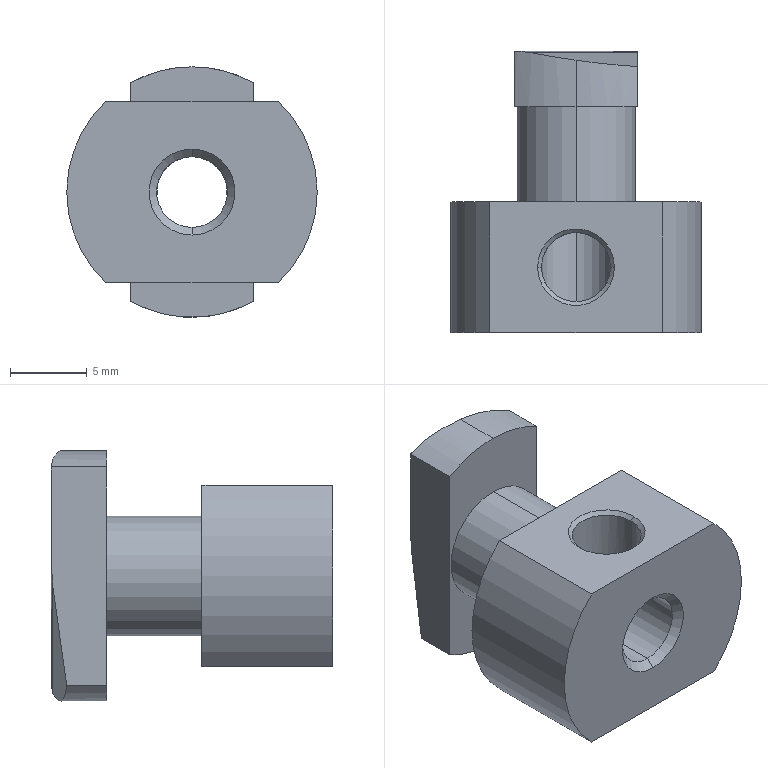Part | SolidWorks | features BaseBody 1 | 1 solid | 27 faces | box 16.3 x 18.3 x 16.3 mm | volume 1833 mm3 | cylinder 13 | plane 10 | cone 4 | commonest cylinder face diameters 16.3 x5 4.5 x2 4.6 x2 7.8 x2 10 x2
STEP:
#1=CARTESIAN_POINT('',(0.,-8.,2.3));
#2=VERTEX_POINT('',#1);
#3=CARTESIAN_POINT('',(0.,-8.,-2.3));
#4=VERTEX_POINT('',#3);
#5=CARTESIAN_POINT('',(0.,-8.,0.));
#6=DIRECTION('',(0.,-1.,0.));
#7=DIRECTION('',(0.,0.,-1.));
#8=AXIS2_PLACEMENT_3D('',#5,#6,#7);
#9=CIRCLE('',#8,2.3);
#10=EDGE_CURVE('',#2,#4,#9,.T.);
#11=ORIENTED_EDGE('',*,*,#10,.F.);
#12=CARTESIAN_POINT('',(0.,-8.5,2.8));
#13=VERTEX_POINT('',#12);
#14=CARTESIAN_POINT('',(0.,-8.5,2.8));
#15=DIRECTION('',(0.,-0.7071,0.7071));
#16=VECTOR('',#15,1000.);
#17=LINE('',#14,#16);
#18=EDGE_CURVE('',#2,#13,#17,.T.);
#19=ORIENTED_EDGE('',*,*,#18,.T.);
#20=CARTESIAN_POINT('',(0.,-8.5,-2.8));
#21=VERTEX_POINT('',#20);
#22=CARTESIAN_POINT('',(0.,-8.5,0.));
#23=DIRECTION('',(0.,-1.,0.));
#24=DIRECTION('',(0.,0.,-1.));
#25=AXIS2_PLACEMENT_3D('',#22,#23,#24);
#26=CIRCLE('',#25,2.8);
#27=EDGE_CURVE('',#13,#21,#26,.T.);
#28=ORIENTED_EDGE('',*,*,#27,.T.);
#29=CARTESIAN_POINT('',(0.,-8.5,-2.8));
#30=DIRECTION('',(0.,-0.7071,-0.7071));
#31=VECTOR('',#30,1000.);
#32=LINE('',#29,#31);
#33=EDGE_CURVE('',#4,#21,#32,.T.);
#34=ORIENTED_EDGE('',*,*,#33,.F.);
#35=EDGE_LOOP('',(#11,#19,#28,#34));
#36=FACE_OUTER_BOUND('',#35,.T.);
#37=CARTESIAN_POINT('',(0.,-8.5,0.));
#38=DIRECTION('',(0.,-1.,0.));
#39=DIRECTION('',(0.,0.,-1.));
#40=AXIS2_PLACEMENT_3D('',#37,#38,#39);
#41=CONICAL_SURFACE('',#40,2.8,0.7854);
#42=ADVANCED_FACE('',(#36),#41,.F.);
#43=CARTESIAN_POINT('',(-2.25,-4.25,5.65));
#44=VERTEX_POINT('',#43);
#45=CARTESIAN_POINT('',(2.25,-4.25,5.65));
#46=VERTEX_POINT('',#45);
#47=CARTESIAN_POINT('',(0.,-4.25,5.65));
#48=DIRECTION('',(0.,0.,1.));
#49=DIRECTION('',(1.,0.,0.));
#50=AXIS2_PLACEMENT_3D('',#47,#48,#49);
#51=CIRCLE('',#50,2.25);
#52=EDGE_CURVE('',#44,#46,#51,.T.);
#53=ORIENTED_EDGE('',*,*,#52,.F.);
#54=CARTESIAN_POINT('',(-2.5,-4.25,5.9));
#55=VERTEX_POINT('',#54);
#56=CARTESIAN_POINT('',(-2.5,-4.25,5.9));
#57=DIRECTION('',(-0.7071,0.,0.7071));
#58=VECTOR('',#57,1000.);
#59=LINE('',#56,#58);
#60=EDGE_CURVE('',#44,#55,#59,.T.);
#61=ORIENTED_EDGE('',*,*,#60,.T.);
#62=CARTESIAN_POINT('',(2.5,-4.25,5.9));
#63=VERTEX_POINT('',#62);
#64=CARTESIAN_POINT('',(0.,-4.25,5.9));
#65=DIRECTION('',(0.,0.,-1.));
#66=DIRECTION('',(1.,0.,0.));
#67=AXIS2_PLACEMENT_3D('',#64,#65,#66);
#68=CIRCLE('',#67,2.5);
#69=EDGE_CURVE('',#63,#55,#68,.T.);
#70=ORIENTED_EDGE('',*,*,#69,.F.);
#71=CARTESIAN_POINT('',(2.5,-4.25,5.9));
#72=DIRECTION('',(0.7071,0.,0.7071));
#73=VECTOR('',#72,1000.);
#74=LINE('',#71,#73);
#75=EDGE_CURVE('',#46,#63,#74,.T.);
#76=ORIENTED_EDGE('',*,*,#75,.F.);
#77=EDGE_LOOP('',(#53,#61,#70,#76));
#78=FACE_OUTER_BOUND('',#77,.T.);
#79=CARTESIAN_POINT('',(0.,-4.25,5.9));
#80=DIRECTION('',(0.,0.,1.));
#81=DIRECTION('',(1.,0.,0.));
#82=AXIS2_PLACEMENT_3D('',#79,#80,#81);
#83=CONICAL_SURFACE('',#82,2.5,0.7854);
#84=ADVANCED_FACE('',(#78),#83,.F.);
#85=CARTESIAN_POINT('',(0.,9.8,2.3));
#86=VERTEX_POINT('',#85);
#87=CARTESIAN_POINT('',(0.,9.8,-2.3));
#88=VERTEX_POINT('',#87);
#89=CARTESIAN_POINT('',(0.,9.8,0.));
#90=DIRECTION('',(0.,-1.,0.));
#91=DIRECTION('',(0.,0.,-1.));
#92=AXIS2_PLACEMENT_3D('',#89,#90,#91);
#93=CIRCLE('',#92,2.3);
#94=EDGE_CURVE('',#86,#88,#93,.T.);
#95=ORIENTED_EDGE('',*,*,#94,.F.);
#96=CARTESIAN_POINT('',(0.,-2.,2.3));
#97=VERTEX_POINT('',#96);
#98=CARTESIAN_POINT('',(0.,-8.5,2.3));
#99=DIRECTION('',(0.,-1.,0.));
#100=VECTOR('',#99,1000.);
#101=LINE('',#98,#100);
#102=EDGE_CURVE('',#86,#97,#101,.T.);
#103=ORIENTED_EDGE('',*,*,#102,.T.);
#104=CARTESIAN_POINT('',(-2.25,-4.25,0.477));
#105=VERTEX_POINT('',#104);
#106=CARTESIAN_POINT('',(-2.25,-4.25,0.477));
#107=CARTESIAN_POINT('',(-2.25,-4.164,0.477));
#108=CARTESIAN_POINT('',(-2.245,-4.081,0.5014));
#109=CARTESIAN_POINT('',(-2.228,-3.927,0.572));
#110=CARTESIAN_POINT('',(-2.216,-3.856,0.6166));
#111=CARTESIAN_POINT('',(-2.173,-3.651,0.7595));
#112=CARTESIAN_POINT('',(-2.134,-3.524,0.8665));
#113=CARTESIAN_POINT('',(-2.035,-3.282,1.077));
#114=CARTESIAN_POINT('',(-1.976,-3.166,1.183));
#115=CARTESIAN_POINT('',(-1.836,-2.942,1.391));
#116=CARTESIAN_POINT('',(-1.754,-2.834,1.494));
#117=CARTESIAN_POINT('',(-1.567,-2.63,1.689));
#118=CARTESIAN_POINT('',(-1.463,-2.535,1.78));
#119=CARTESIAN_POINT('',(-1.229,-2.36,1.949));
#120=CARTESIAN_POINT('',(-1.098,-2.28,2.027));
#121=CARTESIAN_POINT('',(-0.8165,-2.148,2.156));
#122=CARTESIAN_POINT('',(-0.6617,-2.093,2.209));
#123=CARTESIAN_POINT('',(-0.3399,-2.02,2.281));
#124=CARTESIAN_POINT('',(-0.1737,-2.,2.3));
#125=CARTESIAN_POINT('',(0.,-2.,2.3));
#126=B_SPLINE_CURVE_WITH_KNOTS('',3,(#106,#107,#108,#109,#110,#111,#112,#113,#114,#115,#116,#117,#118,#119,#120,#121,#122,#123,#124,#125),.UNSPECIFIED.,.F.,.F.,(4,2,2,2,2,2,2,2,2,4),(0.008129,0.008385,0.00864,0.009152,0.009664,0.01018,0.01069,0.0112,0.01171,0.01222),.UNSPECIFIED.);
#127=EDGE_CURVE('',#105,#97,#126,.T.);
#128=ORIENTED_EDGE('',*,*,#127,.F.);
#129=CARTESIAN_POINT('',(0.,-6.5,2.3));
#130=VERTEX_POINT('',#129);
#131=CARTESIAN_POINT('',(0.,-6.5,2.3));
#132=CARTESIAN_POINT('',(-0.1712,-6.5,2.3));
#133=CARTESIAN_POINT('',(-0.3373,-6.481,2.281));
#134=CARTESIAN_POINT('',(-0.6604,-6.407,2.209));
#135=CARTESIAN_POINT('',(-0.8144,-6.353,2.157));
#136=CARTESIAN_POINT('',(-1.097,-6.22,2.027));
#137=CARTESIAN_POINT('',(-1.228,-6.141,1.95));
#138=CARTESIAN_POINT('',(-1.462,-5.966,1.781));
#139=CARTESIAN_POINT('',(-1.566,-5.871,1.69));
#140=CARTESIAN_POINT('',(-1.848,-5.564,1.396));
#141=CARTESIAN_POINT('',(-1.985,-5.341,1.185));
#142=CARTESIAN_POINT('',(-2.134,-4.976,0.8666));
#143=CARTESIAN_POINT('',(-2.173,-4.849,0.7594));
#144=CARTESIAN_POINT('',(-2.216,-4.643,0.6162));
#145=CARTESIAN_POINT('',(-2.228,-4.572,0.5712));
#146=CARTESIAN_POINT('',(-2.245,-4.418,0.5012));
#147=CARTESIAN_POINT('',(-2.25,-4.336,0.477));
#148=CARTESIAN_POINT('',(-2.25,-4.25,0.477));
#149=B_SPLINE_CURVE_WITH_KNOTS('',3,(#131,#132,#133,#134,#135,#136,#137,#138,#139,#140,#141,#142,#143,#144,#145,#146,#147,#148),.UNSPECIFIED.,.F.,.F.,(4,2,2,2,2,2,2,2,4),(0.004063,0.004571,0.00508,0.005588,0.006096,0.007112,0.007621,0.007875,0.008129),.UNSPECIFIED.);
#150=EDGE_CURVE('',#130,#105,#149,.T.);
#151=ORIENTED_EDGE('',*,*,#150,.F.);
#152=CARTESIAN_POINT('',(0.,-8.5,2.3));
#153=DIRECTION('',(0.,-1.,0.));
#154=VECTOR('',#153,1000.);
#155=LINE('',#152,#154);
#156=EDGE_CURVE('',#130,#2,#155,.T.);
#157=ORIENTED_EDGE('',*,*,#156,.T.);
#158=ORIENTED_EDGE('',*,*,#10,.T.);
#159=CARTESIAN_POINT('',(0.,-8.5,-2.3));
#160=DIRECTION('',(0.,-1.,0.));
#161=VECTOR('',#160,1000.);
#162=LINE('',#159,#161);
#163=EDGE_CURVE('',#88,#4,#162,.T.);
#164=ORIENTED_EDGE('',*,*,#163,.F.);
#165=EDGE_LOOP('',(#95,#103,#128,#151,#157,#158,#164));
#166=FACE_OUTER_BOUND('',#165,.T.);
#167=CARTESIAN_POINT('',(0.,-8.5,0.));
#168=DIRECTION('',(0.,-1.,0.));
#169=DIRECTION('',(0.,0.,-1.));
#170=AXIS2_PLACEMENT_3D('',#167,#168,#169);
#171=CYLINDRICAL_SURFACE('',#170,2.3);
#172=ADVANCED_FACE('',(#166),#171,.F.);
#173=CARTESIAN_POINT('',(0.,0.,-3.9));
#174=VERTEX_POINT('',#173);
#175=CARTESIAN_POINT('',(0.,0.,3.9));
#176=VERTEX_POINT('',#175);
#177=CARTESIAN_POINT('',(0.,0.,0.));
#178=DIRECTION('',(0.,-1.,0.));
#179=DIRECTION('',(0.,0.,1.));
#180=AXIS2_PLACEMENT_3D('',#177,#178,#179);
#181=CIRCLE('',#180,3.9);
#182=EDGE_CURVE('',#174,#176,#181,.T.);
#183=ORIENTED_EDGE('',*,*,#182,.F.);
#184=CARTESIAN_POINT('',(0.,6.2,-3.9));
#185=VERTEX_POINT('',#184);
#186=CARTESIAN_POINT('',(0.,0.,-3.9));
#187=DIRECTION('',(0.,1.,0.));
#188=VECTOR('',#187,1000.);
#189=LINE('',#186,#188);
#190=EDGE_CURVE('',#174,#185,#189,.T.);
#191=ORIENTED_EDGE('',*,*,#190,.T.);
#192=CARTESIAN_POINT('',(0.,6.2,3.9));
#193=VERTEX_POINT('',#192);
#194=CARTESIAN_POINT('',(0.,6.2,0.));
#195=DIRECTION('',(0.,-1.,0.));
#196=DIRECTION('',(0.,0.,1.));
#197=AXIS2_PLACEMENT_3D('',#194,#195,#196);
#198=CIRCLE('',#197,3.9);
#199=EDGE_CURVE('',#185,#193,#198,.T.);
#200=ORIENTED_EDGE('',*,*,#199,.T.);
#201=CARTESIAN_POINT('',(0.,0.,3.9));
#202=DIRECTION('',(0.,1.,0.));
#203=VECTOR('',#202,1000.);
#204=LINE('',#201,#203);
#205=EDGE_CURVE('',#176,#193,#204,.T.);
#206=ORIENTED_EDGE('',*,*,#205,.F.);
#207=EDGE_LOOP('',(#183,#191,#200,#206));
#208=FACE_OUTER_BOUND('',#207,.T.);
#209=CARTESIAN_POINT('',(0.,0.,0.));
#210=DIRECTION('',(0.,1.,0.));
#211=DIRECTION('',(0.,0.,1.));
#212=AXIS2_PLACEMENT_3D('',#209,#210,#211);
#213=CYLINDRICAL_SURFACE('',#212,3.9);
#214=ADVANCED_FACE('',(#208),#213,.T.);
#215=CARTESIAN_POINT('',(2.25,-4.25,0.477));
#216=VERTEX_POINT('',#215);
#217=CARTESIAN_POINT('',(2.25,-4.25,0.477));
#218=CARTESIAN_POINT('',(2.25,-4.336,0.477));
#219=CARTESIAN_POINT('',(2.245,-4.419,0.5014));
#220=CARTESIAN_POINT('',(2.228,-4.573,0.572));
#221=CARTESIAN_POINT('',(2.216,-4.644,0.6166));
#222=CARTESIAN_POINT('',(2.173,-4.849,0.7595));
#223=CARTESIAN_POINT('',(2.134,-4.976,0.8665));
#224=CARTESIAN_POINT('',(2.035,-5.218,1.077));
#225=CARTESIAN_POINT('',(1.976,-5.334,1.183));
#226=CARTESIAN_POINT('',(1.836,-5.558,1.391));
#227=CARTESIAN_POINT('',(1.754,-5.666,1.494));
#228=CARTESIAN_POINT('',(1.567,-5.87,1.689));
#229=CARTESIAN_POINT('',(1.463,-5.965,1.78));
#230=CARTESIAN_POINT('',(1.229,-6.14,1.949));
#231=CARTESIAN_POINT('',(1.098,-6.22,2.027));
#232=CARTESIAN_POINT('',(0.8165,-6.352,2.156));
#233=CARTESIAN_POINT('',(0.6617,-6.407,2.209));
#234=CARTESIAN_POINT('',(0.3399,-6.48,2.281));
#235=CARTESIAN_POINT('',(0.1711,-6.5,2.3));
#236=CARTESIAN_POINT('',(0.,-6.5,2.3));
#237=B_SPLINE_CURVE_WITH_KNOTS('',3,(#217,#218,#219,#220,#221,#222,#223,#224,#225,#226,#227,#228,#229,#230,#231,#232,#233,#234,#235,#236),.UNSPECIFIED.,.F.,.F.,(4,2,2,2,2,2,2,2,2,4),(0.,0.000254,0.0005079,0.001016,0.001524,0.002032,0.00254,0.003047,0.003555,0.004063),.UNSPECIFIED.);
#238=EDGE_CURVE('',#216,#130,#237,.T.);
#239=ORIENTED_EDGE('',*,*,#238,.T.);
#240=ORIENTED_EDGE('',*,*,#150,.T.);
#241=CARTESIAN_POINT('',(-2.25,-4.25,5.9));
#242=DIRECTION('',(0.,0.,1.));
#243=VECTOR('',#242,1000.);
#244=LINE('',#241,#243);
#245=EDGE_CURVE('',#105,#44,#244,.T.);
#246=ORIENTED_EDGE('',*,*,#245,.T.);
#247=ORIENTED_EDGE('',*,*,#52,.T.);
#248=CARTESIAN_POINT('',(2.25,-4.25,5.9));
#249=DIRECTION('',(0.,0.,1.));
#250=VECTOR('',#249,1000.);
#251=LINE('',#248,#250);
#252=EDGE_CURVE('',#216,#46,#251,.T.);
#253=ORIENTED_EDGE('',*,*,#252,.F.);
#254=EDGE_LOOP('',(#239,#240,#246,#247,#253));
#255=FACE_OUTER_BOUND('',#254,.T.);
#256=CARTESIAN_POINT('',(0.,-4.25,5.9));
#257=DIRECTION('',(0.,0.,1.));
#258=DIRECTION('',(1.,0.,0.));
#259=AXIS2_PLACEMENT_3D('',#256,#257,#258);
#260=CYLINDRICAL_SURFACE('',#259,2.25);
#261=ADVANCED_FACE('',(#255),#260,.F.);
#262=CARTESIAN_POINT('',(-4.,6.2,7.101));
#263=VERTEX_POINT('',#262);
#264=CARTESIAN_POINT('',(0.,6.2,8.15));
#265=VERTEX_POINT('',#264);
#266=CARTESIAN_POINT('',(0.,6.2,0.));
#267=DIRECTION('',(0.,1.,0.));
#268=DIRECTION('',(0.,0.,1.));
#269=AXIS2_PLACEMENT_3D('',#266,#267,#268);
#270=CIRCLE('',#269,8.15);
#271=EDGE_CURVE('',#263,#265,#270,.T.);
#272=ORIENTED_EDGE('',*,*,#271,.T.);
#273=CARTESIAN_POINT('',(0.,9.217,8.15));
#274=VERTEX_POINT('',#273);
#275=CARTESIAN_POINT('',(0.,6.2,8.15));
#276=DIRECTION('',(0.,1.,0.));
#277=VECTOR('',#276,1000.);
#278=LINE('',#275,#277);
#279=EDGE_CURVE('',#265,#274,#278,.T.);
#280=ORIENTED_EDGE('',*,*,#279,.T.);
#281=CARTESIAN_POINT('',(-2.9,9.703,7.617));
#282=VERTEX_POINT('',#281);
#283=CARTESIAN_POINT('',(0.,9.217,8.15));
#284=CARTESIAN_POINT('',(-0.9939,9.358,8.15));
#285=CARTESIAN_POINT('',(-1.971,9.522,7.97));
#286=CARTESIAN_POINT('',(-2.9,9.703,7.617));
#287=(BOUNDED_CURVE()B_SPLINE_CURVE(3,(#283,#284,#285,#286),.UNSPECIFIED.,.F.,.T.)B_SPLINE_CURVE_WITH_KNOTS((4,4),(3.927,4.291),.UNSPECIFIED.)CURVE()GEOMETRIC_REPRESENTATION_ITEM()RATIONAL_B_SPLINE_CURVE((1.,0.989,0.989,1.))REPRESENTATION_ITEM(''));
#288=EDGE_CURVE('',#274,#282,#287,.T.);
#289=ORIENTED_EDGE('',*,*,#288,.T.);
#290=CARTESIAN_POINT('',(-3.852,9.8,7.182));
#291=VERTEX_POINT('',#290);
#292=CARTESIAN_POINT('',(-3.852,9.8,7.182));
#293=CARTESIAN_POINT('',(-3.542,9.8,7.349));
#294=CARTESIAN_POINT('',(-3.224,9.766,7.493));
#295=CARTESIAN_POINT('',(-2.9,9.703,7.617));
#296=B_SPLINE_CURVE_WITH_KNOTS('',3,(#292,#293,#294,#295),.UNSPECIFIED.,.F.,.F.,(4,4),(0.,0.001051),.UNSPECIFIED.);
#297=EDGE_CURVE('',#291,#282,#296,.T.);
#298=ORIENTED_EDGE('',*,*,#297,.F.);
#299=CARTESIAN_POINT('',(-4.,9.8,7.101));
#300=VERTEX_POINT('',#299);
#301=CARTESIAN_POINT('',(0.,9.8,0.));
#302=DIRECTION('',(0.,-1.,0.));
#303=DIRECTION('',(0.,0.,1.));
#304=AXIS2_PLACEMENT_3D('',#301,#302,#303);
#305=CIRCLE('',#304,8.15);
#306=EDGE_CURVE('',#291,#300,#305,.T.);
#307=ORIENTED_EDGE('',*,*,#306,.T.);
#308=CARTESIAN_POINT('',(-4.,6.2,7.101));
#309=DIRECTION('',(0.,1.,0.));
#310=VECTOR('',#309,1000.);
#311=LINE('',#308,#310);
#312=EDGE_CURVE('',#263,#300,#311,.T.);
#313=ORIENTED_EDGE('',*,*,#312,.F.);
#314=EDGE_LOOP('',(#272,#280,#289,#298,#307,#313));
#315=FACE_OUTER_BOUND('',#314,.T.);
#316=CARTESIAN_POINT('',(0.,6.2,0.));
#317=DIRECTION('',(0.,1.,0.));
#318=DIRECTION('',(0.,0.,1.));
#319=AXIS2_PLACEMENT_3D('',#316,#317,#318);
#320=CYLINDRICAL_SURFACE('',#319,8.15);
#321=ADVANCED_FACE('',(#315),#320,.T.);
#322=CARTESIAN_POINT('',(-5.622,-8.5,5.9));
#323=VERTEX_POINT('',#322);
#324=CARTESIAN_POINT('',(5.622,-8.5,5.9));
#325=VERTEX_POINT('',#324);
#326=CARTESIAN_POINT('',(0.,-8.5,5.9));
#327=DIRECTION('',(1.,0.,0.));
#328=VECTOR('',#327,1000.);
#329=LINE('',#326,#328);
#330=EDGE_CURVE('',#323,#325,#329,.T.);
#331=ORIENTED_EDGE('',*,*,#330,.F.);
#332=CARTESIAN_POINT('',(-5.622,-8.5,-5.9));
#333=VERTEX_POINT('',#332);
#334=CARTESIAN_POINT('',(0.,-8.5,0.));
#335=DIRECTION('',(0.,1.,0.));
#336=DIRECTION('',(0.,0.,1.));
#337=AXIS2_PLACEMENT_3D('',#334,#335,#336);
#338=CIRCLE('',#337,8.15);
#339=EDGE_CURVE('',#333,#323,#338,.T.);
#340=ORIENTED_EDGE('',*,*,#339,.F.);
#341=CARTESIAN_POINT('',(5.622,-8.5,-5.9));
#342=VERTEX_POINT('',#341);
#343=CARTESIAN_POINT('',(0.,-8.5,-5.9));
#344=DIRECTION('',(-1.,0.,0.));
#345=VECTOR('',#344,1000.);
#346=LINE('',#343,#345);
#347=EDGE_CURVE('',#342,#333,#346,.T.);
#348=ORIENTED_EDGE('',*,*,#347,.F.);
#349=CARTESIAN_POINT('',(0.,-8.5,0.));
#350=DIRECTION('',(0.,1.,0.));
#351=DIRECTION('',(0.,0.,1.));
#352=AXIS2_PLACEMENT_3D('',#349,#350,#351);
#353=CIRCLE('',#352,8.15);
#354=EDGE_CURVE('',#325,#342,#353,.T.);
#355=ORIENTED_EDGE('',*,*,#354,.F.);
#356=EDGE_LOOP('',(#331,#340,#348,#355));
#357=FACE_OUTER_BOUND('',#356,.T.);
#358=CARTESIAN_POINT('',(0.,-8.5,0.));
#359=DIRECTION('',(0.,-1.,0.));
#360=DIRECTION('',(0.,0.,-1.));
#361=AXIS2_PLACEMENT_3D('',#358,#359,#360);
#362=CIRCLE('',#361,2.8);
#363=EDGE_CURVE('',#21,#13,#362,.T.);
#364=ORIENTED_EDGE('',*,*,#363,.F.);
#365=ORIENTED_EDGE('',*,*,#27,.F.);
#366=EDGE_LOOP('',(#364,#365));
#367=FACE_BOUND('',#366,.T.);
#368=CARTESIAN_POINT('',(0.,-8.5,0.));
#369=DIRECTION('',(0.,1.,0.));
#370=DIRECTION('',(0.,0.,1.));
#371=AXIS2_PLACEMENT_3D('',#368,#369,#370);
#372=PLANE('',#371);
#373=ADVANCED_FACE('',(#357,#367),#372,.F.);
#374=CARTESIAN_POINT('',(5.622,0.,5.9));
#375=VERTEX_POINT('',#374);
#376=CARTESIAN_POINT('',(5.622,0.,5.9));
#377=DIRECTION('',(0.,-1.,0.));
#378=VECTOR('',#377,1000.);
#379=LINE('',#376,#378);
#380=EDGE_CURVE('',#375,#325,#379,.T.);
#381=ORIENTED_EDGE('',*,*,#380,.T.);
#382=ORIENTED_EDGE('',*,*,#354,.T.);
#383=CARTESIAN_POINT('',(5.622,0.,-5.9));
#384=VERTEX_POINT('',#383);
#385=CARTESIAN_POINT('',(5.622,0.,-5.9));
#386=DIRECTION('',(0.,1.,0.));
#387=VECTOR('',#386,1000.);
#388=LINE('',#385,#387);
#389=EDGE_CURVE('',#342,#384,#388,.T.);
#390=ORIENTED_EDGE('',*,*,#389,.T.);
#391=CARTESIAN_POINT('',(0.,0.,0.));
#392=DIRECTION('',(0.,-1.,0.));
#393=DIRECTION('',(0.,0.,1.));
#394=AXIS2_PLACEMENT_3D('',#391,#392,#393);
#395=CIRCLE('',#394,8.15);
#396=EDGE_CURVE('',#384,#375,#395,.T.);
#397=ORIENTED_EDGE('',*,*,#396,.T.);
#398=EDGE_LOOP('',(#381,#382,#390,#397));
#399=FACE_OUTER_BOUND('',#398,.T.);
#400=CARTESIAN_POINT('',(0.,0.,0.));
#401=DIRECTION('',(0.,1.,0.));
#402=DIRECTION('',(0.,0.,1.));
#403=AXIS2_PLACEMENT_3D('',#400,#401,#402);
#404=CYLINDRICAL_SURFACE('',#403,8.15);
#405=ADVANCED_FACE('',(#399),#404,.T.);
#406=CARTESIAN_POINT('',(-5.622,0.,5.9));
#407=VERTEX_POINT('',#406);
#408=CARTESIAN_POINT('',(-5.622,0.,5.9));
#409=DIRECTION('',(0.,-1.,0.));
#410=VECTOR('',#409,1000.);
#411=LINE('',#408,#410);
#412=EDGE_CURVE('',#407,#323,#411,.T.);
#413=ORIENTED_EDGE('',*,*,#412,.T.);
#414=ORIENTED_EDGE('',*,*,#330,.T.);
#415=ORIENTED_EDGE('',*,*,#380,.F.);
#416=CARTESIAN_POINT('',(-5.622,0.,5.9));
#417=DIRECTION('',(-1.,0.,0.));
#418=VECTOR('',#417,1000.);
#419=LINE('',#416,#418);
#420=EDGE_CURVE('',#375,#407,#419,.T.);
#421=ORIENTED_EDGE('',*,*,#420,.T.);
#422=EDGE_LOOP('',(#413,#414,#415,#421));
#423=FACE_OUTER_BOUND('',#422,.T.);
#424=ORIENTED_EDGE('',*,*,#69,.T.);
#425=CARTESIAN_POINT('',(0.,-4.25,5.9));
#426=DIRECTION('',(0.,0.,-1.));
#427=DIRECTION('',(1.,0.,0.));
#428=AXIS2_PLACEMENT_3D('',#425,#426,#427);
#429=CIRCLE('',#428,2.5);
#430=EDGE_CURVE('',#55,#63,#429,.T.);
#431=ORIENTED_EDGE('',*,*,#430,.T.);
#432=EDGE_LOOP('',(#424,#431));
#433=FACE_BOUND('',#432,.T.);
#434=CARTESIAN_POINT('',(-5.622,0.,5.9));
#435=DIRECTION('',(0.,0.,1.));
#436=DIRECTION('',(1.,0.,0.));
#437=AXIS2_PLACEMENT_3D('',#434,#435,#436);
#438=PLANE('',#437);
#439=ADVANCED_FACE('',(#423,#433),#438,.T.);
#440=CARTESIAN_POINT('',(-5.622,0.,-5.9));
#441=VERTEX_POINT('',#440);
#442=CARTESIAN_POINT('',(-5.622,0.,-5.9));
#443=DIRECTION('',(0.,-1.,0.));
#444=VECTOR('',#443,1000.);
#445=LINE('',#442,#444);
#446=EDGE_CURVE('',#441,#333,#445,.T.);
#447=ORIENTED_EDGE('',*,*,#446,.T.);
#448=ORIENTED_EDGE('',*,*,#339,.T.);
#449=ORIENTED_EDGE('',*,*,#412,.F.);
#450=CARTESIAN_POINT('',(0.,0.,0.));
#451=DIRECTION('',(0.,-1.,0.));
#452=DIRECTION('',(0.,0.,1.));
#453=AXIS2_PLACEMENT_3D('',#450,#451,#452);
#454=CIRCLE('',#453,8.15);
#455=EDGE_CURVE('',#407,#441,#454,.T.);
#456=ORIENTED_EDGE('',*,*,#455,.T.);
#457=EDGE_LOOP('',(#447,#448,#449,#456));
#458=FACE_OUTER_BOUND('',#457,.T.);
#459=CARTESIAN_POINT('',(0.,0.,0.));
#460=DIRECTION('',(0.,1.,0.));
#461=DIRECTION('',(0.,0.,1.));
#462=AXIS2_PLACEMENT_3D('',#459,#460,#461);
#463=CYLINDRICAL_SURFACE('',#462,8.15);
#464=ADVANCED_FACE('',(#458),#463,.T.);
#465=ORIENTED_EDGE('',*,*,#389,.F.);
#466=ORIENTED_EDGE('',*,*,#347,.T.);
#467=ORIENTED_EDGE('',*,*,#446,.F.);
#468=CARTESIAN_POINT('',(5.622,0.,-5.9));
#469=DIRECTION('',(1.,0.,0.));
#470=VECTOR('',#469,1000.);
#471=LINE('',#468,#470);
#472=EDGE_CURVE('',#441,#384,#471,.T.);
#473=ORIENTED_EDGE('',*,*,#472,.T.);
#474=EDGE_LOOP('',(#465,#466,#467,#473));
#475=FACE_OUTER_BOUND('',#474,.T.);
#476=CARTESIAN_POINT('',(5.622,0.,-5.9));
#477=DIRECTION('',(0.,0.,-1.));
#478=DIRECTION('',(-1.,0.,0.));
#479=AXIS2_PLACEMENT_3D('',#476,#477,#478);
#480=PLANE('',#479);
#481=ADVANCED_FACE('',(#475),#480,.T.);
#482=ORIENTED_EDGE('',*,*,#18,.F.);
#483=CARTESIAN_POINT('',(0.,-8.,0.));
#484=DIRECTION('',(0.,-1.,0.));
#485=DIRECTION('',(0.,0.,-1.));
#486=AXIS2_PLACEMENT_3D('',#483,#484,#485);
#487=CIRCLE('',#486,2.3);
#488=EDGE_CURVE('',#4,#2,#487,.T.);
#489=ORIENTED_EDGE('',*,*,#488,.F.);
#490=ORIENTED_EDGE('',*,*,#33,.T.);
#491=ORIENTED_EDGE('',*,*,#363,.T.);
#492=EDGE_LOOP('',(#482,#489,#490,#491));
#493=FACE_OUTER_BOUND('',#492,.T.);
#494=CARTESIAN_POINT('',(0.,-8.5,0.));
#495=DIRECTION('',(0.,-1.,0.));
#496=DIRECTION('',(0.,0.,-1.));
#497=AXIS2_PLACEMENT_3D('',#494,#495,#496);
#498=CONICAL_SURFACE('',#497,2.8,0.7854);
#499=ADVANCED_FACE('',(#493),#498,.F.);
#500=ORIENTED_EDGE('',*,*,#420,.F.);
#501=ORIENTED_EDGE('',*,*,#396,.F.);
#502=ORIENTED_EDGE('',*,*,#472,.F.);
#503=ORIENTED_EDGE('',*,*,#455,.F.);
#504=EDGE_LOOP('',(#500,#501,#502,#503));
#505=FACE_OUTER_BOUND('',#504,.T.);
#506=CARTESIAN_POINT('',(0.,0.,0.));
#507=DIRECTION('',(0.,-1.,0.));
#508=DIRECTION('',(0.,0.,1.));
#509=AXIS2_PLACEMENT_3D('',#506,#507,#508);
#510=CIRCLE('',#509,3.9);
#511=EDGE_CURVE('',#176,#174,#510,.T.);
#512=ORIENTED_EDGE('',*,*,#511,.T.);
#513=ORIENTED_EDGE('',*,*,#182,.T.);
#514=EDGE_LOOP('',(#512,#513));
#515=FACE_BOUND('',#514,.T.);
#516=CARTESIAN_POINT('',(0.,0.,0.));
#517=DIRECTION('',(0.,1.,0.));
#518=DIRECTION('',(0.,0.,1.));
#519=AXIS2_PLACEMENT_3D('',#516,#517,#518);
#520=PLANE('',#519);
#521=ADVANCED_FACE('',(#505,#515),#520,.T.);
#522=ORIENTED_EDGE('',*,*,#60,.F.);
#523=CARTESIAN_POINT('',(0.,-4.25,5.65));
#524=DIRECTION('',(0.,0.,1.));
#525=DIRECTION('',(1.,0.,0.));
#526=AXIS2_PLACEMENT_3D('',#523,#524,#525);
#527=CIRCLE('',#526,2.25);
#528=EDGE_CURVE('',#46,#44,#527,.T.);
#529=ORIENTED_EDGE('',*,*,#528,.F.);
#530=ORIENTED_EDGE('',*,*,#75,.T.);
#531=ORIENTED_EDGE('',*,*,#430,.F.);
#532=EDGE_LOOP('',(#522,#529,#530,#531));
#533=FACE_OUTER_BOUND('',#532,.T.);
#534=CARTESIAN_POINT('',(0.,-4.25,5.9));
#535=DIRECTION('',(0.,0.,1.));
#536=DIRECTION('',(1.,0.,0.));
#537=AXIS2_PLACEMENT_3D('',#534,#535,#536);
#538=CONICAL_SURFACE('',#537,2.5,0.7854);
#539=ADVANCED_FACE('',(#533),#538,.F.);
#540=ORIENTED_EDGE('',*,*,#102,.F.);
#541=CARTESIAN_POINT('',(0.,9.8,0.));
#542=DIRECTION('',(0.,-1.,0.));
#543=DIRECTION('',(0.,0.,-1.));
#544=AXIS2_PLACEMENT_3D('',#541,#542,#543);
#545=CIRCLE('',#544,2.3);
#546=EDGE_CURVE('',#88,#86,#545,.T.);
#547=ORIENTED_EDGE('',*,*,#546,.F.);
#548=ORIENTED_EDGE('',*,*,#163,.T.);
#549=ORIENTED_EDGE('',*,*,#488,.T.);
#550=ORIENTED_EDGE('',*,*,#156,.F.);
#551=ORIENTED_EDGE('',*,*,#238,.F.);
#552=CARTESIAN_POINT('',(0.,-2.,2.3));
#553=CARTESIAN_POINT('',(0.1712,-2.,2.3));
#554=CARTESIAN_POINT('',(0.3373,-2.019,2.281));
#555=CARTESIAN_POINT('',(0.6604,-2.093,2.209));
#556=CARTESIAN_POINT('',(0.8144,-2.147,2.157));
#557=CARTESIAN_POINT('',(1.097,-2.28,2.027));
#558=CARTESIAN_POINT('',(1.228,-2.359,1.95));
#559=CARTESIAN_POINT('',(1.462,-2.534,1.781));
#560=CARTESIAN_POINT('',(1.566,-2.629,1.69));
#561=CARTESIAN_POINT('',(1.848,-2.936,1.396));
#562=CARTESIAN_POINT('',(1.985,-3.159,1.185));
#563=CARTESIAN_POINT('',(2.134,-3.524,0.8666));
#564=CARTESIAN_POINT('',(2.173,-3.651,0.7594));
#565=CARTESIAN_POINT('',(2.216,-3.857,0.6162));
#566=CARTESIAN_POINT('',(2.228,-3.928,0.5712));
#567=CARTESIAN_POINT('',(2.245,-4.082,0.5012));
#568=CARTESIAN_POINT('',(2.25,-4.164,0.477));
#569=CARTESIAN_POINT('',(2.25,-4.25,0.477));
#570=B_SPLINE_CURVE_WITH_KNOTS('',3,(#552,#553,#554,#555,#556,#557,#558,#559,#560,#561,#562,#563,#564,#565,#566,#567,#568,#569),.UNSPECIFIED.,.F.,.F.,(4,2,2,2,2,2,2,2,4),(-0.004035,-0.00353,-0.003026,-0.002522,-0.002017,-0.001009,-0.0005043,-0.0002522,0.),.UNSPECIFIED.);
#571=EDGE_CURVE('',#97,#216,#570,.T.);
#572=ORIENTED_EDGE('',*,*,#571,.F.);
#573=EDGE_LOOP('',(#540,#547,#548,#549,#550,#551,#572));
#574=FACE_OUTER_BOUND('',#573,.T.);
#575=CARTESIAN_POINT('',(0.,-8.5,0.));
#576=DIRECTION('',(0.,-1.,0.));
#577=DIRECTION('',(0.,0.,-1.));
#578=AXIS2_PLACEMENT_3D('',#575,#576,#577);
#579=CYLINDRICAL_SURFACE('',#578,2.3);
#580=ADVANCED_FACE('',(#574),#579,.F.);
#581=ORIENTED_EDGE('',*,*,#190,.F.);
#582=ORIENTED_EDGE('',*,*,#511,.F.);
#583=ORIENTED_EDGE('',*,*,#205,.T.);
#584=CARTESIAN_POINT('',(0.,6.2,0.));
#585=DIRECTION('',(0.,-1.,0.));
#586=DIRECTION('',(0.,0.,1.));
#587=AXIS2_PLACEMENT_3D('',#584,#585,#586);
#588=CIRCLE('',#587,3.9);
#589=EDGE_CURVE('',#193,#185,#588,.T.);
#590=ORIENTED_EDGE('',*,*,#589,.T.);
#591=EDGE_LOOP('',(#581,#582,#583,#590));
#592=FACE_OUTER_BOUND('',#591,.T.);
#593=CARTESIAN_POINT('',(0.,0.,0.));
#594=DIRECTION('',(0.,1.,0.));
#595=DIRECTION('',(0.,0.,1.));
#596=AXIS2_PLACEMENT_3D('',#593,#594,#595);
#597=CYLINDRICAL_SURFACE('',#596,3.9);
#598=ADVANCED_FACE('',(#592),#597,.T.);
#599=ORIENTED_EDGE('',*,*,#245,.F.);
#600=ORIENTED_EDGE('',*,*,#127,.T.);
#601=ORIENTED_EDGE('',*,*,#571,.T.);
#602=ORIENTED_EDGE('',*,*,#252,.T.);
#603=ORIENTED_EDGE('',*,*,#528,.T.);
#604=EDGE_LOOP('',(#599,#600,#601,#602,#603));
#605=FACE_OUTER_BOUND('',#604,.T.);
#606=CARTESIAN_POINT('',(0.,-4.25,5.9));
#607=DIRECTION('',(0.,0.,1.));
#608=DIRECTION('',(1.,0.,0.));
#609=AXIS2_PLACEMENT_3D('',#606,#607,#608);
#610=CYLINDRICAL_SURFACE('',#609,2.25);
#611=ADVANCED_FACE('',(#605),#610,.F.);
#612=CARTESIAN_POINT('',(4.,9.8,-0.6704));
#613=VERTEX_POINT('',#612);
#614=CARTESIAN_POINT('',(-3.852,9.8,7.182));
#615=DIRECTION('',(0.7071,0.,-0.7071));
#616=VECTOR('',#615,1000.);
#617=LINE('',#614,#616);
#618=EDGE_CURVE('',#291,#613,#617,.T.);
#619=ORIENTED_EDGE('',*,*,#618,.T.);
#620=CARTESIAN_POINT('',(4.,9.8,-7.101));
#621=VERTEX_POINT('',#620);
#622=CARTESIAN_POINT('',(4.,9.8,0.));
#623=DIRECTION('',(0.,0.,-1.));
#624=VECTOR('',#623,1000.);
#625=LINE('',#622,#624);
#626=EDGE_CURVE('',#613,#621,#625,.T.);
#627=ORIENTED_EDGE('',*,*,#626,.T.);
#628=CARTESIAN_POINT('',(3.852,9.8,-7.182));
#629=VERTEX_POINT('',#628);
#630=CARTESIAN_POINT('',(0.,9.8,0.));
#631=DIRECTION('',(0.,-1.,0.));
#632=DIRECTION('',(0.,0.,1.));
#633=AXIS2_PLACEMENT_3D('',#630,#631,#632);
#634=CIRCLE('',#633,8.15);
#635=EDGE_CURVE('',#629,#621,#634,.T.);
#636=ORIENTED_EDGE('',*,*,#635,.F.);
#637=CARTESIAN_POINT('',(-4.,9.8,0.6704));
#638=VERTEX_POINT('',#637);
#639=CARTESIAN_POINT('',(3.852,9.8,-7.182));
#640=DIRECTION('',(-0.7071,0.,0.7071));
#641=VECTOR('',#640,1000.);
#642=LINE('',#639,#641);
#643=EDGE_CURVE('',#629,#638,#642,.T.);
#644=ORIENTED_EDGE('',*,*,#643,.T.);
#645=CARTESIAN_POINT('',(-4.,9.8,0.));
#646=DIRECTION('',(0.,0.,1.));
#647=VECTOR('',#646,1000.);
#648=LINE('',#645,#647);
#649=EDGE_CURVE('',#638,#300,#648,.T.);
#650=ORIENTED_EDGE('',*,*,#649,.T.);
#651=ORIENTED_EDGE('',*,*,#306,.F.);
#652=EDGE_LOOP('',(#619,#627,#636,#644,#650,#651));
#653=FACE_OUTER_BOUND('',#652,.T.);
#654=ORIENTED_EDGE('',*,*,#546,.T.);
#655=ORIENTED_EDGE('',*,*,#94,.T.);
#656=EDGE_LOOP('',(#654,#655));
#657=FACE_BOUND('',#656,.T.);
#658=CARTESIAN_POINT('',(0.,9.8,0.));
#659=DIRECTION('',(0.,1.,0.));
#660=DIRECTION('',(0.,0.,1.));
#661=AXIS2_PLACEMENT_3D('',#658,#659,#660);
#662=PLANE('',#661);
#663=ADVANCED_FACE('',(#653,#657),#662,.T.);
#664=CARTESIAN_POINT('',(-4.,6.2,-7.101));
#665=VERTEX_POINT('',#664);
#666=CARTESIAN_POINT('',(-4.,6.2,0.));
#667=DIRECTION('',(0.,0.,1.));
#668=VECTOR('',#667,1000.);
#669=LINE('',#666,#668);
#670=EDGE_CURVE('',#665,#263,#669,.T.);
#671=ORIENTED_EDGE('',*,*,#670,.F.);
#672=CARTESIAN_POINT('',(4.,6.2,-7.101));
#673=VERTEX_POINT('',#672);
#674=CARTESIAN_POINT('',(0.,6.2,0.));
#675=DIRECTION('',(0.,1.,0.));
#676=DIRECTION('',(0.,0.,1.));
#677=AXIS2_PLACEMENT_3D('',#674,#675,#676);
#678=CIRCLE('',#677,8.15);
#679=EDGE_CURVE('',#673,#665,#678,.T.);
#680=ORIENTED_EDGE('',*,*,#679,.F.);
#681=CARTESIAN_POINT('',(4.,6.2,7.101));
#682=VERTEX_POINT('',#681);
#683=CARTESIAN_POINT('',(4.,6.2,0.));
#684=DIRECTION('',(0.,0.,-1.));
#685=VECTOR('',#684,1000.);
#686=LINE('',#683,#685);
#687=EDGE_CURVE('',#682,#673,#686,.T.);
#688=ORIENTED_EDGE('',*,*,#687,.F.);
#689=CARTESIAN_POINT('',(0.,6.2,0.));
#690=DIRECTION('',(0.,1.,0.));
#691=DIRECTION('',(0.,0.,1.));
#692=AXIS2_PLACEMENT_3D('',#689,#690,#691);
#693=CIRCLE('',#692,8.15);
#694=EDGE_CURVE('',#265,#682,#693,.T.);
#695=ORIENTED_EDGE('',*,*,#694,.F.);
#696=ORIENTED_EDGE('',*,*,#271,.F.);
#697=EDGE_LOOP('',(#671,#680,#688,#695,#696));
#698=FACE_OUTER_BOUND('',#697,.T.);
#699=ORIENTED_EDGE('',*,*,#589,.F.);
#700=ORIENTED_EDGE('',*,*,#199,.F.);
#701=EDGE_LOOP('',(#699,#700));
#702=FACE_BOUND('',#701,.T.);
#703=CARTESIAN_POINT('',(0.,6.2,0.));
#704=DIRECTION('',(0.,1.,0.));
#705=DIRECTION('',(0.,0.,1.));
#706=AXIS2_PLACEMENT_3D('',#703,#704,#705);
#707=PLANE('',#706);
#708=ADVANCED_FACE('',(#698,#702),#707,.F.);
#709=ORIENTED_EDGE('',*,*,#687,.T.);
#710=CARTESIAN_POINT('',(4.,6.2,-7.101));
#711=DIRECTION('',(0.,1.,0.));
#712=VECTOR('',#711,1000.);
#713=LINE('',#710,#712);
#714=EDGE_CURVE('',#673,#621,#713,.T.);
#715=ORIENTED_EDGE('',*,*,#714,.T.);
#716=ORIENTED_EDGE('',*,*,#626,.F.);
#717=CARTESIAN_POINT('',(4.,9.703,0.7164));
#718=VERTEX_POINT('',#717);
#719=CARTESIAN_POINT('',(4.,9.8,-0.6704));
#720=CARTESIAN_POINT('',(4.,9.8,-0.2043));
#721=CARTESIAN_POINT('',(4.,9.768,0.2594));
#722=CARTESIAN_POINT('',(4.,9.703,0.7164));
#723=(BOUNDED_CURVE()B_SPLINE_CURVE(3,(#719,#720,#721,#722),.UNSPECIFIED.,.F.,.F.)B_SPLINE_CURVE_WITH_KNOTS((4,4),(1.571,1.768),.UNSPECIFIED.)CURVE()GEOMETRIC_REPRESENTATION_ITEM()RATIONAL_B_SPLINE_CURVE((1.,0.9968,0.9968,1.))REPRESENTATION_ITEM(''));
#724=EDGE_CURVE('',#613,#718,#723,.T.);
#725=ORIENTED_EDGE('',*,*,#724,.T.);
#726=CARTESIAN_POINT('',(4.,8.8,7.101));
#727=VERTEX_POINT('',#726);
#728=CARTESIAN_POINT('',(4.,9.703,0.7164));
#729=DIRECTION('',(0.,-0.14,0.9901));
#730=VECTOR('',#729,1000.);
#731=LINE('',#728,#730);
#732=EDGE_CURVE('',#718,#727,#731,.T.);
#733=ORIENTED_EDGE('',*,*,#732,.T.);
#734=CARTESIAN_POINT('',(4.,6.2,7.101));
#735=DIRECTION('',(0.,-1.,0.));
#736=VECTOR('',#735,1000.);
#737=LINE('',#734,#736);
#738=EDGE_CURVE('',#727,#682,#737,.T.);
#739=ORIENTED_EDGE('',*,*,#738,.T.);
#740=EDGE_LOOP('',(#709,#715,#716,#725,#733,#739));
#741=FACE_OUTER_BOUND('',#740,.T.);
#742=CARTESIAN_POINT('',(4.,6.2,7.101));
#743=DIRECTION('',(1.,0.,0.));
#744=DIRECTION('',(0.,0.,-1.));
#745=AXIS2_PLACEMENT_3D('',#742,#743,#744);
#746=PLANE('',#745);
#747=ADVANCED_FACE('',(#741),#746,.T.);
#748=ORIENTED_EDGE('',*,*,#618,.F.);
#749=ORIENTED_EDGE('',*,*,#297,.T.);
#750=CARTESIAN_POINT('',(-28.729,9.703,33.445));
#751=DIRECTION('',(0.7071,0.,-0.7071));
#752=VECTOR('',#751,1000.);
#753=LINE('',#750,#752);
#754=EDGE_CURVE('',#282,#718,#753,.T.);
#755=ORIENTED_EDGE('',*,*,#754,.T.);
#756=ORIENTED_EDGE('',*,*,#724,.F.);
#757=EDGE_LOOP('',(#748,#749,#755,#756));
#758=FACE_OUTER_BOUND('',#757,.T.);
#759=CARTESIAN_POINT('',(-29.422,4.8,32.752));
#760=DIRECTION('',(0.7071,0.,-0.7071));
#761=DIRECTION('',(-0.7071,0.,-0.7071));
#762=AXIS2_PLACEMENT_3D('',#759,#760,#761);
#763=CYLINDRICAL_SURFACE('',#762,5.);
#764=ADVANCED_FACE('',(#758),#763,.T.);
#765=ORIENTED_EDGE('',*,*,#670,.T.);
#766=ORIENTED_EDGE('',*,*,#312,.T.);
#767=ORIENTED_EDGE('',*,*,#649,.F.);
#768=CARTESIAN_POINT('',(-4.,9.703,-0.7164));
#769=VERTEX_POINT('',#768);
#770=CARTESIAN_POINT('',(-4.,9.8,0.6704));
#771=CARTESIAN_POINT('',(-4.,9.8,0.2043));
#772=CARTESIAN_POINT('',(-4.,9.768,-0.2594));
#773=CARTESIAN_POINT('',(-4.,9.703,-0.7164));
#774=(BOUNDED_CURVE()B_SPLINE_CURVE(3,(#770,#771,#772,#773),.UNSPECIFIED.,.F.,.T.)B_SPLINE_CURVE_WITH_KNOTS((4,4),(1.571,1.768),.UNSPECIFIED.)CURVE()GEOMETRIC_REPRESENTATION_ITEM()RATIONAL_B_SPLINE_CURVE((1.,0.9968,0.9968,1.))REPRESENTATION_ITEM(''));
#775=EDGE_CURVE('',#638,#769,#774,.T.);
#776=ORIENTED_EDGE('',*,*,#775,.T.);
#777=CARTESIAN_POINT('',(-4.,8.8,-7.101));
#778=VERTEX_POINT('',#777);
#779=CARTESIAN_POINT('',(-4.,9.703,-0.7164));
#780=DIRECTION('',(0.,-0.14,-0.9901));
#781=VECTOR('',#780,1000.);
#782=LINE('',#779,#781);
#783=EDGE_CURVE('',#769,#778,#782,.T.);
#784=ORIENTED_EDGE('',*,*,#783,.T.);
#785=CARTESIAN_POINT('',(-4.,6.2,-7.101));
#786=DIRECTION('',(0.,-1.,0.));
#787=VECTOR('',#786,1000.);
#788=LINE('',#785,#787);
#789=EDGE_CURVE('',#778,#665,#788,.T.);
#790=ORIENTED_EDGE('',*,*,#789,.T.);
#791=EDGE_LOOP('',(#765,#766,#767,#776,#784,#790));
#792=FACE_OUTER_BOUND('',#791,.T.);
#793=CARTESIAN_POINT('',(-4.,6.2,-7.101));
#794=DIRECTION('',(-1.,0.,0.));
#795=DIRECTION('',(0.,0.,1.));
#796=AXIS2_PLACEMENT_3D('',#793,#794,#795);
#797=PLANE('',#796);
#798=ADVANCED_FACE('',(#792),#797,.T.);
#799=ORIENTED_EDGE('',*,*,#643,.F.);
#800=CARTESIAN_POINT('',(2.9,9.703,-7.617));
#801=VERTEX_POINT('',#800);
#802=CARTESIAN_POINT('',(3.852,9.8,-7.182));
#803=CARTESIAN_POINT('',(3.542,9.8,-7.349));
#804=CARTESIAN_POINT('',(3.224,9.766,-7.493));
#805=CARTESIAN_POINT('',(2.9,9.703,-7.617));
#806=B_SPLINE_CURVE_WITH_KNOTS('',3,(#802,#803,#804,#805),.UNSPECIFIED.,.F.,.F.,(4,4),(0.,0.001051),.UNSPECIFIED.);
#807=EDGE_CURVE('',#629,#801,#806,.T.);
#808=ORIENTED_EDGE('',*,*,#807,.T.);
#809=CARTESIAN_POINT('',(28.729,9.703,-33.445));
#810=DIRECTION('',(-0.7071,0.,0.7071));
#811=VECTOR('',#810,1000.);
#812=LINE('',#809,#811);
#813=EDGE_CURVE('',#801,#769,#812,.T.);
#814=ORIENTED_EDGE('',*,*,#813,.T.);
#815=ORIENTED_EDGE('',*,*,#775,.F.);
#816=EDGE_LOOP('',(#799,#808,#814,#815));
#817=FACE_OUTER_BOUND('',#816,.T.);
#818=CARTESIAN_POINT('',(29.422,4.8,-32.752));
#819=DIRECTION('',(-0.7071,0.,0.7071));
#820=DIRECTION('',(0.7071,0.,0.7071));
#821=AXIS2_PLACEMENT_3D('',#818,#819,#820);
#822=CYLINDRICAL_SURFACE('',#821,5.);
#823=ADVANCED_FACE('',(#817),#822,.T.);
#824=ORIENTED_EDGE('',*,*,#279,.F.);
#825=ORIENTED_EDGE('',*,*,#694,.T.);
#826=ORIENTED_EDGE('',*,*,#738,.F.);
#827=CARTESIAN_POINT('',(4.,8.8,7.101));
#828=CARTESIAN_POINT('',(2.772,8.876,7.792));
#829=CARTESIAN_POINT('',(1.409,9.018,8.15));
#830=CARTESIAN_POINT('',(0.,9.217,8.15));
#831=(BOUNDED_CURVE()B_SPLINE_CURVE(3,(#827,#828,#829,#830),.UNSPECIFIED.,.F.,.T.)B_SPLINE_CURVE_WITH_KNOTS((4,4),(3.414,3.927),.UNSPECIFIED.)CURVE()GEOMETRIC_REPRESENTATION_ITEM()RATIONAL_B_SPLINE_CURVE((1.,0.9782,0.9782,1.))REPRESENTATION_ITEM(''));
#832=EDGE_CURVE('',#727,#274,#831,.T.);
#833=ORIENTED_EDGE('',*,*,#832,.T.);
#834=EDGE_LOOP('',(#824,#825,#826,#833));
#835=FACE_OUTER_BOUND('',#834,.T.);
#836=CARTESIAN_POINT('',(0.,6.2,0.));
#837=DIRECTION('',(0.,1.,0.));
#838=DIRECTION('',(0.,0.,1.));
#839=AXIS2_PLACEMENT_3D('',#836,#837,#838);
#840=CYLINDRICAL_SURFACE('',#839,8.15);
#841=ADVANCED_FACE('',(#835),#840,.T.);
#842=ORIENTED_EDGE('',*,*,#679,.T.);
#843=ORIENTED_EDGE('',*,*,#789,.F.);
#844=CARTESIAN_POINT('',(-4.,8.8,-7.101));
#845=CARTESIAN_POINT('',(-1.855,8.932,-8.309));
#846=CARTESIAN_POINT('',(0.5996,9.254,-8.493));
#847=CARTESIAN_POINT('',(2.9,9.703,-7.617));
#848=(BOUNDED_CURVE()B_SPLINE_CURVE(3,(#844,#845,#846,#847),.UNSPECIFIED.,.F.,.T.)B_SPLINE_CURVE_WITH_KNOTS((4,4),(3.414,4.291),.UNSPECIFIED.)CURVE()GEOMETRIC_REPRESENTATION_ITEM()RATIONAL_B_SPLINE_CURVE((1.,0.937,0.937,1.))REPRESENTATION_ITEM(''));
#849=EDGE_CURVE('',#778,#801,#848,.T.);
#850=ORIENTED_EDGE('',*,*,#849,.T.);
#851=ORIENTED_EDGE('',*,*,#807,.F.);
#852=ORIENTED_EDGE('',*,*,#635,.T.);
#853=ORIENTED_EDGE('',*,*,#714,.F.);
#854=EDGE_LOOP('',(#842,#843,#850,#851,#852,#853));
#855=FACE_OUTER_BOUND('',#854,.T.);
#856=CARTESIAN_POINT('',(0.,6.2,0.));
#857=DIRECTION('',(0.,1.,0.));
#858=DIRECTION('',(0.,0.,1.));
#859=AXIS2_PLACEMENT_3D('',#856,#857,#858);
#860=CYLINDRICAL_SURFACE('',#859,8.15);
#861=ADVANCED_FACE('',(#855),#860,.T.);
#862=ORIENTED_EDGE('',*,*,#832,.F.);
#863=ORIENTED_EDGE('',*,*,#732,.F.);
#864=ORIENTED_EDGE('',*,*,#754,.F.);
#865=ORIENTED_EDGE('',*,*,#288,.F.);
#866=EDGE_LOOP('',(#862,#863,#864,#865));
#867=FACE_OUTER_BOUND('',#866,.T.);
#868=CARTESIAN_POINT('',(10.147,9.8,-6.117));
#869=DIRECTION('',(0.1387,0.9806,0.1387));
#870=DIRECTION('',(0.,-0.14,0.9901));
#871=AXIS2_PLACEMENT_3D('',#868,#869,#870);
#872=PLANE('',#871);
#873=ADVANCED_FACE('',(#867),#872,.T.);
#874=ORIENTED_EDGE('',*,*,#813,.F.);
#875=ORIENTED_EDGE('',*,*,#849,.F.);
#876=ORIENTED_EDGE('',*,*,#783,.F.);
#877=EDGE_LOOP('',(#874,#875,#876));
#878=FACE_OUTER_BOUND('',#877,.T.);
#879=CARTESIAN_POINT('',(6.117,9.8,-10.147));
#880=DIRECTION('',(0.1387,-0.9806,0.1387));
#881=DIRECTION('',(0.,-0.14,-0.9901));
#882=AXIS2_PLACEMENT_3D('',#879,#880,#881);
#883=PLANE('',#882);
#884=ADVANCED_FACE('',(#878),#883,.F.);
#885=CLOSED_SHELL('',(#42,#84,#172,#214,#261,#321,#373,#405,#439,#464,#481,#499,#521,#539,#580,#598,#611,#663,#708,#747,#764,#798,#823,#841,#861,#873,#884));
#886=MANIFOLD_SOLID_BREP('',#885);
#887=CARTESIAN_POINT('',(0.,0.,0.));
#888=DIRECTION('',(0.,0.,1.));
#889=DIRECTION('',(1.,0.,0.));
#890=AXIS2_PLACEMENT_3D('',#887,#888,#889);
#891=(LENGTH_UNIT()NAMED_UNIT(*)SI_UNIT(.MILLI.,.METRE.));
#892=UNCERTAINTY_MEASURE_WITH_UNIT(LENGTH_MEASURE(0.00001),#891,'','');
#893=(NAMED_UNIT(*)PLANE_ANGLE_UNIT()SI_UNIT($,.RADIAN.));
#894=(NAMED_UNIT(*)SI_UNIT($,.STERADIAN.)SOLID_ANGLE_UNIT());
#895=(GEOMETRIC_REPRESENTATION_CONTEXT(3)GLOBAL_UNCERTAINTY_ASSIGNED_CONTEXT((#892))GLOBAL_UNIT_ASSIGNED_CONTEXT((#891,#893,#894))REPRESENTATION_CONTEXT('',''));
#896=ADVANCED_BREP_SHAPE_REPRESENTATION('',(#886,#890),#895);